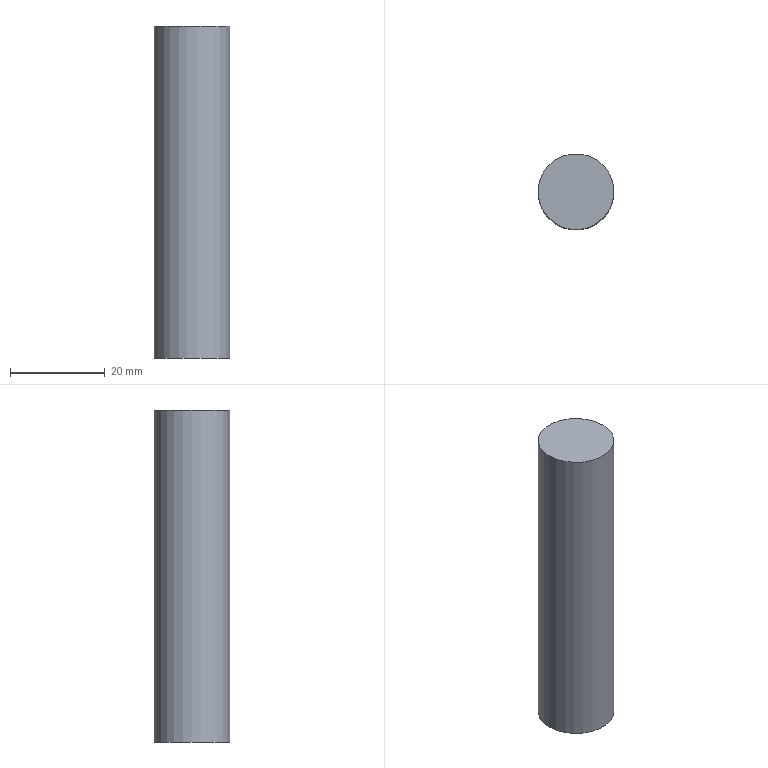Part | STEP file | solid 214 | 1 solid | 3 faces | box 16 x 16 x 70 mm | volume 14074 mm3 | plane 2 | cylinder 1 | commonest cylinder face diameters 16 x1